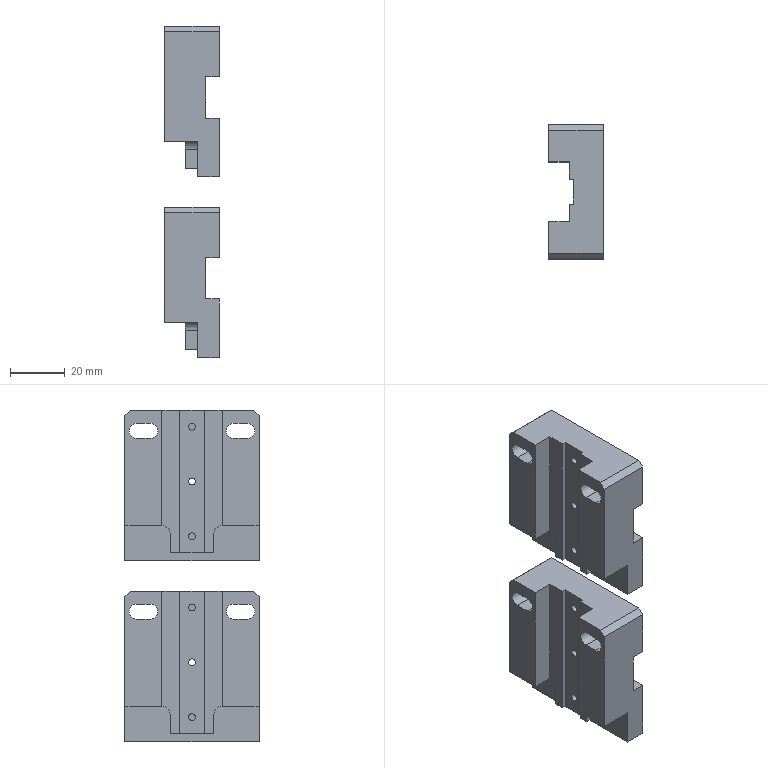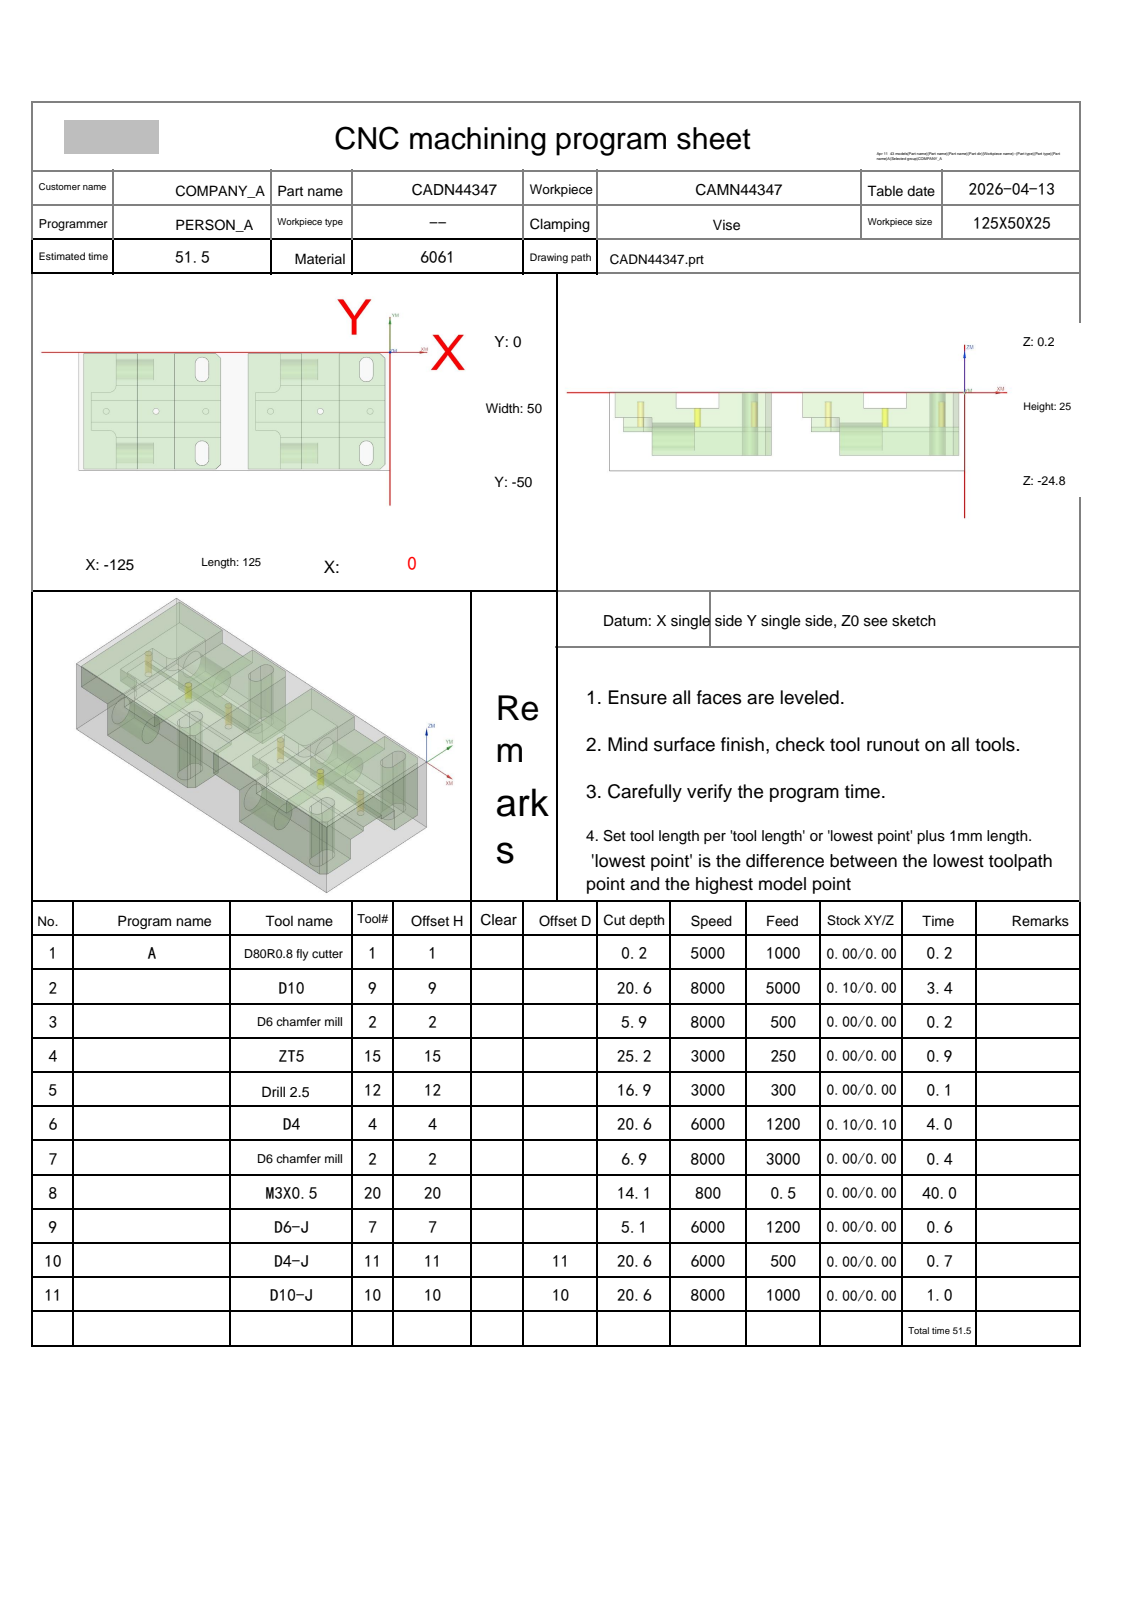NC program | NX | posted by the shop | part box 19.9 x 49 x 121 mm
Lines 3110 to 3925 of 3925:
N7 T02 M06
(D6 chamfer mill  D=6. R=0. H=02 ce=0.00 di=0.00)
G00 G90 G54 X-22.578 Y-25.25 M03 S8000
G43 H02 Z20.
M08
Z2.099
G01 Z-1.5 F3000.
G03 X-22.278 Y-25.33 I.3 J.52
X-21.758 Y-25.03 I0.0 J.6
G01 X-21.75 Y-25.
Y-.5
G02 X-20.45 Y.8 I1.3 J0.0
G01 X-4.
X-3.746 Y.775
X-3.503 Y.701
X-3.278 Y.581
X-3.081 Y.419
X-1.081 Y-1.581
X-.919 Y-1.778
X-.799 Y-2.003
X-.725 Y-2.246
X-.7 Y-2.5
Y-47.5
X-.725 Y-47.754
X-.799 Y-47.997
X-.919 Y-48.222
X-1.081 Y-48.419
X-3.081 Y-50.419
X-3.278 Y-50.581
X-3.503 Y-50.701
X-3.746 Y-50.775
X-4. Y-50.8
X-20.45
G02 X-21.75 Y-49.5 I0.0 J1.3
G01 Y-25.
X-21.758 Y-24.97
G03 X-22.278 Y-24.67 I-.52 J-.3
X-22.578 Y-24.75 I0.0 J-.6
G01 Z2.099
G00 Z20.
X-10.122 Y-42.5
Z2.099
G01 Z-1.5
G03 X-10.422 Y-42.42 I-.3 J-.52
X-10.942 Y-42.72 I0.0 J-.6
G01 X-10.95 Y-42.75
Y-45.25
G03 X-9.5 Y-46.7 I1.45 J0.0
X-8.05 Y-45.25 I0.0 J1.45
G01 Y-40.25
G03 X-9.5 Y-38.8 I-1.45 J0.0
X-10.95 Y-40.25 I0.0 J-1.45
G01 Y-42.75
X-10.942 Y-42.78
G03 X-10.422 Y-43.08 I.52 J.3
X-10.122 Y-43. I0.0 J.6
G01 Z2.099
G00 Z20.
Y-7.
Z2.099
G01 Z-1.5
G03 X-10.422 Y-6.92 I-.3 J-.52
X-10.942 Y-7.22 I0.0 J-.6
G01 X-10.95 Y-7.25
Y-9.75
G03 X-9.5 Y-11.2 I1.45 J0.0
X-8.05 Y-9.75 I0.0 J1.45
G01 Y-4.75
G03 X-9.5 Y-3.3 I-1.45 J0.0
X-10.95 Y-4.75 I0.0 J-1.45
G01 Y-7.25
X-10.942 Y-7.28
G03 X-10.422 Y-7.58 I.52 J.3
X-10.122 Y-7.5 I0.0 J.6
G01 Z2.099
G00 Z20.
X-59.128 Y-25.25
Z2.099
G01 Z-1.5
G03 X-58.828 Y-25.33 I.3 J.52
X-58.308 Y-25.03 I0.0 J.6
G01 X-58.3 Y-25.
Y-.5
G02 X-57. Y.8 I1.3 J0.0
G01 X-35.55
G02 X-34.25 Y-.5 I0.0 J-1.3
G01 Y-49.5
G02 X-35.55 Y-50.8 I-1.3 J0.0
G01 X-57.
G02 X-58.3 Y-49.5 I0.0 J1.3
G01 Y-25.
X-58.308 Y-24.97
G03 X-58.828 Y-24.67 I-.52 J-.3
X-59.128 Y-24.75 I0.0 J-.6
G01 Z2.099
G00 Z20.
X-88.578 Y-25.25
Z2.099
G01 Z-1.5
G03 X-88.278 Y-25.33 I.3 J.52
X-87.758 Y-25.03 I0.0 J.6
G01 X-87.75 Y-25.
Y-.5
G02 X-86.45 Y.8 I1.3 J0.0
G01 X-70.
X-69.746 Y.775
X-69.503 Y.701
X-69.278 Y.581
X-69.081 Y.419
X-67.081 Y-1.581
X-66.919 Y-1.778
X-66.799 Y-2.003
X-66.725 Y-2.246
X-66.7 Y-2.5
Y-47.5
X-66.725 Y-47.754
X-66.799 Y-47.997
X-66.919 Y-48.222
X-67.081 Y-48.419
X-69.081 Y-50.419
X-69.278 Y-50.581
X-69.503 Y-50.701
X-69.746 Y-50.775
X-70. Y-50.8
X-86.45
G02 X-87.75 Y-49.5 I0.0 J1.3
G01 Y-25.
X-87.758 Y-24.97
G03 X-88.278 Y-24.67 I-.52 J-.3
X-88.578 Y-24.75 I0.0 J-.6
G01 Z2.099
G00 Z20.
X-76.122 Y-42.5
Z2.099
G01 Z-1.5
G03 X-76.422 Y-42.42 I-.3 J-.52
X-76.942 Y-42.72 I0.0 J-.6
G01 X-76.95 Y-42.75
Y-45.25
G03 X-75.5 Y-46.7 I1.45 J0.0
X-74.05 Y-45.25 I0.0 J1.45
G01 Y-40.25
G03 X-75.5 Y-38.8 I-1.45 J0.0
X-76.95 Y-40.25 I0.0 J-1.45
G01 Y-42.75
X-76.942 Y-42.78
G03 X-76.422 Y-43.08 I.52 J.3
X-76.122 Y-43. I0.0 J.6
G01 Z2.099
G00 Z20.
Y-7.
Z2.099
G01 Z-1.5
G03 X-76.422 Y-6.92 I-.3 J-.52
X-76.942 Y-7.22 I0.0 J-.6
G01 X-76.95 Y-7.25
Y-9.75
G03 X-75.5 Y-11.2 I1.45 J0.0
X-74.05 Y-9.75 I0.0 J1.45
G01 Y-4.75
G03 X-75.5 Y-3.3 I-1.45 J0.0
X-76.95 Y-4.75 I0.0 J-1.45
G01 Y-7.25
X-76.942 Y-7.28
G03 X-76.422 Y-7.58 I.52 J.3
X-76.122 Y-7.5 I0.0 J.6
G01 Z2.099
G00 Z20.
X-125.128 Y-25.25
Z2.099
G01 Z-1.5
G03 X-124.828 Y-25.33 I.3 J.52
X-124.308 Y-25.03 I0.0 J.6
G01 X-124.3 Y-25.
Y-.5
G02 X-123. Y.8 I1.3 J0.0
G01 X-101.55
G02 X-100.25 Y-.5 I0.0 J-1.3
G01 Y-49.5
G02 X-101.55 Y-50.8 I-1.3 J0.0
G01 X-123.
G02 X-124.3 Y-49.5 I0.0 J1.3
G01 Y-25.
X-124.308 Y-24.97
G03 X-124.828 Y-24.67 I-.52 J-.3
X-125.128 Y-24.75 I0.0 J-.6
G01 Z2.099
G00 Z20.
X-98.501 Y1.545
Z1.755
G01 Z-6.4
G03 X-98.573 Y1.275 I.468 J-.27
X-98.303 Y.807 I.54 J0.0
G01 X-98.276 Y.8
X-89.724
X-89.697 Y.807
G03 X-89.427 Y1.275 I-.27 J.468
X-89.499 Y1.545 I-.54 J0.0
G01 Z1.755
G00 Z20.
Y-51.545
Z1.755
G01 Z-6.4
G03 X-89.427 Y-51.275 I-.468 J.27
X-89.697 Y-50.807 I-.54 J0.0
G01 X-89.724 Y-50.8
X-98.276
X-98.303 Y-50.807
G03 X-98.573 Y-51.275 I.27 J-.468
X-98.501 Y-51.545 I.54 J0.0
G01 Z1.755
G00 Z20.
X-32.501 Y1.545
Z1.755
G01 Z-6.4
G03 X-32.573 Y1.275 I.468 J-.27
X-32.303 Y.807 I.54 J0.0
G01 X-32.276 Y.8
X-23.724
X-23.697 Y.807
G03 X-23.427 Y1.275 I-.27 J.468
X-23.499 Y1.545 I-.54 J0.0
G01 Z1.755
G00 Z20.
Y-51.545
Z1.755
G01 Z-6.4
G03 X-23.427 Y-51.275 I-.468 J.27
X-23.697 Y-50.807 I-.54 J0.0
G01 X-23.724 Y-50.8
X-32.276
X-32.303 Y-50.807
G03 X-32.573 Y-51.275 I.27 J-.468
X-32.501 Y-51.545 I.54 J0.0
G01 Z1.755
G00 Z20.
G00 G90 X-28. Y-25. M03 S8000
Z20.
G98 G81 X-28. Y-25. Z-6.65 R-1.9 F500.
X-94.
G80
G00 Z20.
G91 G28 Z0.0
M05
M09
G91 G28 Z0.0
M01
N8 T20 M06
(M3X0.5 D=2.5 DR_a=180 H=20)
G00 G90 G54 X-28. Y-25. M03 S800
G43 H20 Z20.
M08
G95
G98 G84 X-28. Y-25. Z-13.9 R-3.9 F.5 Q5.
X-94.
G80
G94
G00 Z20.
G91 G28 Z0.0
M05
M09
G91 G28 Z0.0
M01
N9 T07 M06
(D6-J  D=6. R=0. H=07 ce=0.30 di=0.00)
G00 G90 G54 X-23.751 Y5.8 M03 S6000
G43 H07 Z20.
M08
Z-4.4
G01 Z-4.9 F1200.
Y2.5
Y-52.5
X-26.584
Y2.5
X-29.417
Y-52.5
X-32.25
Y2.5
Y5.8
Z-4.4
G00 Z20.
X-89.751
Z-4.4
G01 Z-4.9
Y2.5
Y-52.5
X-92.584
Y2.5
X-95.417
Y-52.5
X-98.25
Y2.5
Y5.8
Z-4.4
G00 Z20.
G00 G90 X-31.45 Y3.2 M03 S6000
Z20.
Z-4.395
G01 Z-4.895 F1200.
G41 D07
X-31.55
G03 X-32.55 Y2.2 I0.0 J-1.
G01 Y-52.2
G03 X-31.55 Y-53.2 I1. J0.0
G01 G40 X-31.45
Z-4.395
G00 Z20.
X-24.55
Z-4.395
G01 Z-4.895
G41 D07
X-24.45
G03 X-23.45 Y-52.2 I0.0 J1.
G01 Y2.2
G03 X-24.45 Y3.2 I-1. J0.0
G01 G40 X-24.55
Z-4.395
G00 Z20.
X-97.45
Z-4.395
G01 Z-4.895
G41 D07
X-97.55
G03 X-98.55 Y2.2 I0.0 J-1.
G01 Y-52.2
G03 X-97.55 Y-53.2 I1. J0.0
G01 G40 X-97.45
Z-4.395
G00 Z20.
X-90.55
Z-4.395
G01 Z-4.895
G41 D07
X-90.45
G03 X-89.45 Y-52.2 I0.0 J1.
G01 Y2.2
G03 X-90.45 Y3.2 I-1. J0.0
G01 G40 X-90.55
Z-4.395
G00 Z20.
G91 G28 Z0.0
M05
M09
G91 G28 Z0.0
M01
N10 T11 M06
(D4-J  D=4. R=0. H=11 ce=0.00 di=0.00)
G00 G90 G54 X-10. Y-42.55 M03 S6000
G43 H11 Z20.
M08
Z-3.58
G01 Z-4.08 F500.
G41 D11
X-10.05
G03 X-10.25 Y-42.75 I0.0 J-.2
G01 Y-45.25
G03 X-9.5 Y-46. I.75 J0.0
X-8.75 Y-45.25 I0.0 J.75
G01 Y-40.25
G03 X-9.5 Y-39.5 I-.75 J0.0
X-10.25 Y-40.25 I0.0 J-.75
G01 Y-42.75
Y-43.25
G03 X-10.05 Y-43.45 I.2 J0.0
G01 G40 X-10.
Z-3.58
G00 Z1.
Y-42.55
Z-7.66
G01 Z-8.16
G41 D11
X-10.05
G03 X-10.25 Y-42.75 I0.0 J-.2
G01 Y-45.25
G03 X-9.5 Y-46. I.75 J0.0
X-8.75 Y-45.25 I0.0 J.75
G01 Y-40.25
G03 X-9.5 Y-39.5 I-.75 J0.0
X-10.25 Y-40.25 I0.0 J-.75
G01 Y-42.75
Y-43.25
G03 X-10.05 Y-43.45 I.2 J0.0
G01 G40 X-10.
Z-7.66
G00 Z-3.08
Y-42.55
Z-11.74
G01 Z-12.24
G41 D11
X-10.05
G03 X-10.25 Y-42.75 I0.0 J-.2
G01 Y-45.25
G03 X-9.5 Y-46. I.75 J0.0
X-8.75 Y-45.25 I0.0 J.75
G01 Y-40.25
G03 X-9.5 Y-39.5 I-.75 J0.0
X-10.25 Y-40.25 I0.0 J-.75
G01 Y-42.75
Y-43.25
G03 X-10.05 Y-43.45 I.2 J0.0
G01 G40 X-10.
Z-11.74
G00 Z-7.16
Y-42.55
Z-15.82
G01 Z-16.32
G41 D11
X-10.05
G03 X-10.25 Y-42.75 I0.0 J-.2
G01 Y-45.25
G03 X-9.5 Y-46. I.75 J0.0
X-8.75 Y-45.25 I0.0 J.75
G01 Y-40.25
G03 X-9.5 Y-39.5 I-.75 J0.0
X-10.25 Y-40.25 I0.0 J-.75
G01 Y-42.75
Y-43.25
G03 X-10.05 Y-43.45 I.2 J0.0
G01 G40 X-10.
Z-15.82
G00 Z-11.24
Y-42.55
Z-19.9
G01 Z-20.4
G41 D11
X-10.05
G03 X-10.25 Y-42.75 I0.0 J-.2
G01 Y-45.25
G03 X-9.5 Y-46. I.75 J0.0
X-8.75 Y-45.25 I0.0 J.75
G01 Y-40.25
G03 X-9.5 Y-39.5 I-.75 J0.0
X-10.25 Y-40.25 I0.0 J-.75
G01 Y-42.75
Y-43.25
G03 X-10.05 Y-43.45 I.2 J0.0
G01 G40 X-10.
Z-19.9
G00 Z20.
X-9. Y-7.45
Z-3.58
G01 Z-4.08
G41 D11
X-8.95
G03 X-8.75 Y-7.25 I0.0 J.2
G01 Y-4.75
G03 X-9.5 Y-4. I-.75 J0.0
X-10.25 Y-4.75 I0.0 J-.75
G01 Y-9.75
G03 X-9.5 Y-10.5 I.75 J0.0
X-8.75 Y-9.75 I0.0 J.75
G01 Y-7.25
Y-6.75
G03 X-8.95 Y-6.55 I-.2 J0.0
G01 G40 X-9.
Z-3.58
G00 Z1.
Y-7.45
Z-7.66
G01 Z-8.16
G41 D11
X-8.95
G03 X-8.75 Y-7.25 I0.0 J.2
G01 Y-4.75
G03 X-9.5 Y-4. I-.75 J0.0
X-10.25 Y-4.75 I0.0 J-.75
G01 Y-9.75
G03 X-9.5 Y-10.5 I.75 J0.0
X-8.75 Y-9.75 I0.0 J.75
G01 Y-7.25
Y-6.75
G03 X-8.95 Y-6.55 I-.2 J0.0
G01 G40 X-9.
Z-7.66
G00 Z-3.08
Y-7.45
Z-11.74
G01 Z-12.24
G41 D11
X-8.95
G03 X-8.75 Y-7.25 I0.0 J.2
G01 Y-4.75
G03 X-9.5 Y-4. I-.75 J0.0
X-10.25 Y-4.75 I0.0 J-.75
G01 Y-9.75
G03 X-9.5 Y-10.5 I.75 J0.0
X-8.75 Y-9.75 I0.0 J.75
G01 Y-7.25
Y-6.75
G03 X-8.95 Y-6.55 I-.2 J0.0
G01 G40 X-9.
Z-11.74
G00 Z-7.16
Y-7.45
Z-15.82
G01 Z-16.32
G41 D11
X-8.95
G03 X-8.75 Y-7.25 I0.0 J.2
G01 Y-4.75
G03 X-9.5 Y-4. I-.75 J0.0
X-10.25 Y-4.75 I0.0 J-.75
G01 Y-9.75
G03 X-9.5 Y-10.5 I.75 J0.0
X-8.75 Y-9.75 I0.0 J.75
G01 Y-7.25
Y-6.75
G03 X-8.95 Y-6.55 I-.2 J0.0
G01 G40 X-9.
Z-15.82
G00 Z-11.24
Y-7.45
Z-19.9
G01 Z-20.4
G41 D11
X-8.95
G03 X-8.75 Y-7.25 I0.0 J.2
G01 Y-4.75
G03 X-9.5 Y-4. I-.75 J0.0
X-10.25 Y-4.75 I0.0 J-.75
G01 Y-9.75
G03 X-9.5 Y-10.5 I.75 J0.0
X-8.75 Y-9.75 I0.0 J.75
G01 Y-7.25
Y-6.75
G03 X-8.95 Y-6.55 I-.2 J0.0
G01 G40 X-9.
Z-19.9
G00 Z20.
X-75. Y-7.45
Z-3.58
G01 Z-4.08
G41 D11
X-74.95
G03 X-74.75 Y-7.25 I0.0 J.2
G01 Y-4.75
G03 X-75.5 Y-4. I-.75 J0.0
X-76.25 Y-4.75 I0.0 J-.75
G01 Y-9.75
G03 X-75.5 Y-10.5 I.75 J0.0
X-74.75 Y-9.75 I0.0 J.75
G01 Y-7.25
Y-6.75
G03 X-74.95 Y-6.55 I-.2 J0.0
G01 G40 X-75.
Z-3.58
G00 Z1.
Y-7.45
Z-7.66
G01 Z-8.16
G41 D11
X-74.95
G03 X-74.75 Y-7.25 I0.0 J.2
G01 Y-4.75
G03 X-75.5 Y-4. I-.75 J0.0
X-76.25 Y-4.75 I0.0 J-.75
G01 Y-9.75
G03 X-75.5 Y-10.5 I.75 J0.0
X-74.75 Y-9.75 I0.0 J.75
G01 Y-7.25
Y-6.75
G03 X-74.95 Y-6.55 I-.2 J0.0
G01 G40 X-75.
Z-7.66
G00 Z-3.08
Y-7.45
Z-11.74
G01 Z-12.24
G41 D11
X-74.95
G03 X-74.75 Y-7.25 I0.0 J.2
G01 Y-4.75
G03 X-75.5 Y-4. I-.75 J0.0
X-76.25 Y-4.75 I0.0 J-.75
G01 Y-9.75
G03 X-75.5 Y-10.5 I.75 J0.0
X-74.75 Y-9.75 I0.0 J.75
G01 Y-7.25
Y-6.75
G03 X-74.95 Y-6.55 I-.2 J0.0
G01 G40 X-75.
Z-11.74
G00 Z-7.16
Y-7.45
Z-15.82
G01 Z-16.32
G41 D11
X-74.95
G03 X-74.75 Y-7.25 I0.0 J.2
G01 Y-4.75
G03 X-75.5 Y-4. I-.75 J0.0
X-76.25 Y-4.75 I0.0 J-.75
G01 Y-9.75
G03 X-75.5 Y-10.5 I.75 J0.0
X-74.75 Y-9.75 I0.0 J.75
G01 Y-7.25
Y-6.75
G03 X-74.95 Y-6.55 I-.2 J0.0
G01 G40 X-75.
Z-15.82
G00 Z-11.24
Y-7.45
Z-19.9
G01 Z-20.4
G41 D11
X-74.95
G03 X-74.75 Y-7.25 I0.0 J.2
G01 Y-4.75
G03 X-75.5 Y-4. I-.75 J0.0
X-76.25 Y-4.75 I0.0 J-.75
G01 Y-9.75
G03 X-75.5 Y-10.5 I.75 J0.0
X-74.75 Y-9.75 I0.0 J.75
G01 Y-7.25
Y-6.75
G03 X-74.95 Y-6.55 I-.2 J0.0
G01 G40 X-75.
Z-19.9
G00 Z20.
Y-42.95
Z-3.58
G01 Z-4.08
G41 D11
X-74.95
G03 X-74.75 Y-42.75 I0.0 J.2
G01 Y-40.25
G03 X-75.5 Y-39.5 I-.75 J0.0
X-76.25 Y-40.25 I0.0 J-.75
G01 Y-45.25
G03 X-75.5 Y-46. I.75 J0.0
X-74.75 Y-45.25 I0.0 J.75
G01 Y-42.75
Y-42.25
G03 X-74.95 Y-42.05 I-.2 J0.0
G01 G40 X-75.
Z-3.58
G00 Z1.
Y-42.95
Z-7.66
G01 Z-8.16
G41 D11
X-74.95
G03 X-74.75 Y-42.75 I0.0 J.2
G01 Y-40.25
G03 X-75.5 Y-39.5 I-.75 J0.0
X-76.25 Y-40.25 I0.0 J-.75
G01 Y-45.25
G03 X-75.5 Y-46. I.75 J0.0
X-74.75 Y-45.25 I0.0 J.75
G01 Y-42.75
Y-42.25
G03 X-74.95 Y-42.05 I-.2 J0.0
G01 G40 X-75.
Z-7.66
G00 Z-3.08
Y-42.95
Z-11.74
G01 Z-12.24
G41 D11
X-74.95
G03 X-74.75 Y-42.75 I0.0 J.2
G01 Y-40.25
G03 X-75.5 Y-39.5 I-.75 J0.0
X-76.25 Y-40.25 I0.0 J-.75
G01 Y-45.25
G03 X-75.5 Y-46. I.75 J0.0
X-74.75 Y-45.25 I0.0 J.75
G01 Y-42.75
Y-42.25
G03 X-74.95 Y-42.05 I-.2 J0.0
G01 G40 X-75.
Z-11.74
G00 Z-7.16
Y-42.95
Z-15.82
G01 Z-16.32
G41 D11
X-74.95
G03 X-74.75 Y-42.75 I0.0 J.2
G01 Y-40.25
G03 X-75.5 Y-39.5 I-.75 J0.0
X-76.25 Y-40.25 I0.0 J-.75
G01 Y-45.25
G03 X-75.5 Y-46. I.75 J0.0
X-74.75 Y-45.25 I0.0 J.75
G01 Y-42.75
Y-42.25
G03 X-74.95 Y-42.05 I-.2 J0.0
G01 G40 X-75.
Z-15.82
G00 Z-11.24
Y-42.95
Z-19.9
G01 Z-20.4
G41 D11
X-74.95
G03 X-74.75 Y-42.75 I0.0 J.2
G01 Y-40.25
G03 X-75.5 Y-39.5 I-.75 J0.0
X-76.25 Y-40.25 I0.0 J-.75
G01 Y-45.25
G03 X-75.5 Y-46. I.75 J0.0
X-74.75 Y-45.25 I0.0 J.75
G01 Y-42.75
Y-42.25
G03 X-74.95 Y-42.05 I-.2 J0.0
G01 G40 X-75.
Z-19.9
G00 Z20.
G91 G28 Z0.0
M05
M09
G91 G28 Z0.0
M01
N11 T10 M06
(D10-J  D=10. R=0. H=10 ce=0.00 di=0.00)
G00 G90 G54 X-2.987 Y-55.616 M03 S8000
G43 H10 Z20.
M08
Z-9.7
G01 Z-10.2 F1000.
G41 D10
X-3.003 Y-55.417
G03 X-4. Y-54.5 I-.997 J-.083
G01 X-57.
G02 X-62. Y-49.501 I0.0 J5.
G01 Y-.499
G02 X-57. Y4.5 I5. J-.001
G01 X-4.
G02 X-.464 Y3.036 I0.0 J-5.
G01 X1.536 Y1.036
G02 X3. Y-2.5 I-3.536 J-3.536
G01 Y-47.5
G02 X1.536 Y-51.036 I-5. J0.0
G01 X-.464 Y-53.036
G02 X-4. Y-54.5 I-3.536 J3.536
G01 X-4.5
G03 X-5.5 Y-55.5 I0.0 J-1.
G01 G40 Y-55.7
Z-9.7
G00 Z20.
X-95.5
Z-9.7
G01 Z-10.2
G41 D10
Y-55.5
G03 X-96.5 Y-54.5 I-1. J0.0
G01 X-123.
G02 X-128. Y-49.5 I0.0 J5.
G01 Y-.5
G02 X-123. Y4.5 I5. J0.0
G01 X-70.
G02 X-66.464 Y3.036 I0.0 J-5.
G01 X-64.464 Y1.036
G02 X-63. Y-2.5 I-3.536 J-3.536
G01 Y-47.5
G02 X-64.464 Y-51.036 I-5. J0.0
G01 X-66.464 Y-53.036
G02 X-70. Y-54.5 I-3.536 J3.536
G01 X-96.5
X-97.
G03 X-98. Y-55.5 I0.0 J-1.
G01 G40 Y-55.7
Z-9.7
G00 Z20.
X-68.987 Y-55.616
Z-19.9
G01 Z-20.4
G41 D10
X-69.003 Y-55.417
G03 X-70. Y-54.5 I-.997 J-.083
G01 X-123.
G02 X-128. Y-49.5 I0.0 J5.
G01 Y-.5
G02 X-123. Y4.5 I5. J0.0
G01 X-70.
G02 X-66.464 Y3.036 I0.0 J-5.
G01 X-64.464 Y1.036
G02 X-63. Y-2.5 I-3.536 J-3.536
G01 Y-47.5
G02 X-64.464 Y-51.036 I-5. J0.0
G01 X-66.464 Y-53.036
G02 X-70. Y-54.5 I-3.536 J3.536
G01 X-70.5
G03 X-71.5 Y-55.5 I0.0 J-1.
G01 G40 Y-55.7
X-62.345 Y-52.641
G41 D10
X-62.165 Y-52.554
G03 X-61.6 Y-51.654 I-.436 J.9
X-61.667 Y-51.295 I-1. J0.0
G02 X-62. Y-49.503 I4.667 J1.795
G01 Y-.499
G02 X-57. Y4.5 I5. J-.001
G01 X-4.
G02 X-.464 Y3.036 I0.0 J-5.
G01 X1.536 Y1.036
G02 X3. Y-2.5 I-3.536 J-3.536
G01 Y-47.5
G02 X1.536 Y-51.036 I-5. J0.0
G01 X-.464 Y-53.036
G02 X-4. Y-54.5 I-3.536 J3.536
G01 X-57.
G02 X-61.667 Y-51.295 I0.0 J5.
X-61.823 Y-50.82 I4.667 J1.795
G03 X-62.787 Y-50.084 I-.965 J-.264
X-63.051 Y-50.12 I0.0 J-1.
G01 G40 X-62.89 Y-50.644
Z-19.9
G00 Z20.
M05
M09
G91 G28 Z0.0
G91 G28 Y0.0
M30
%